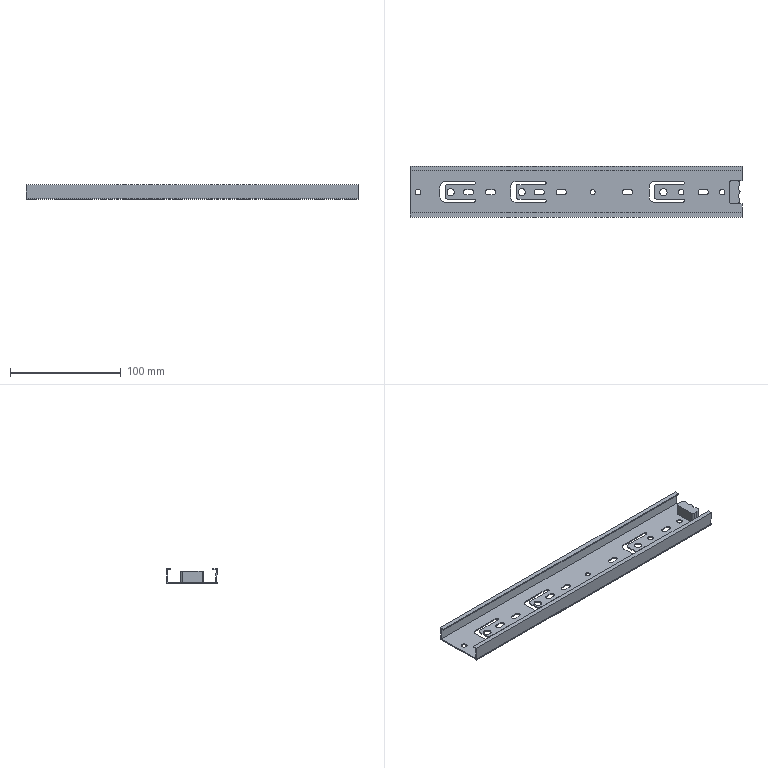Part | STEP file | slide rail 300-1 | 3 solids | 105 faces | box 300 x 46.341 x 13 mm | volume 22910 mm3 | plane 61 | cylinder 42 | spline 2 | commonest cylinder face diameters 3 x17 4.6 x12 10 x6 5 x3 6.5 x3 4.5 x1